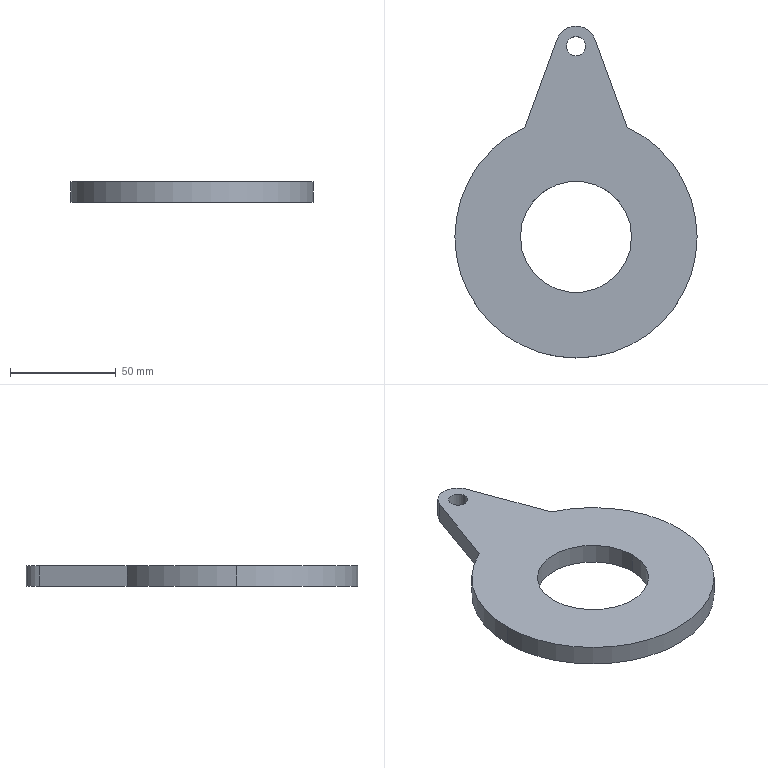Part | SolidWorks | features Extrusion 1 | 1 solid | 12 faces | box 114.3 x 156.675 x 9.525 mm | volume 88657 mm3 | cylinder 8 | plane 4 | commonest cylinder face diameters 114.3 x3 9 x2 52.502 x2 19.05 x1
STEP:
#1=CARTESIAN_POINT('',(-4.5,90.,231.775));
#2=VERTEX_POINT('',#1);
#3=CARTESIAN_POINT('',(4.5,90.,231.775));
#4=VERTEX_POINT('',#3);
#5=CARTESIAN_POINT('',(0.,90.,231.775));
#6=DIRECTION('',(0.,0.,1.));
#7=DIRECTION('',(1.,0.,0.));
#8=AXIS2_PLACEMENT_3D('',#5,#6,#7);
#9=CIRCLE('',#8,4.5);
#10=EDGE_CURVE('',#2,#4,#9,.T.);
#11=ORIENTED_EDGE('',*,*,#10,.T.);
#12=CARTESIAN_POINT('',(4.5,90.,222.25));
#13=VERTEX_POINT('',#12);
#14=CARTESIAN_POINT('',(4.5,90.,231.775));
#15=DIRECTION('',(0.,0.,-1.));
#16=VECTOR('',#15,1000.);
#17=LINE('',#14,#16);
#18=EDGE_CURVE('',#4,#13,#17,.T.);
#19=ORIENTED_EDGE('',*,*,#18,.T.);
#20=CARTESIAN_POINT('',(-4.5,90.,222.25));
#21=VERTEX_POINT('',#20);
#22=CARTESIAN_POINT('',(0.,90.,222.25));
#23=DIRECTION('',(0.,0.,1.));
#24=DIRECTION('',(1.,0.,0.));
#25=AXIS2_PLACEMENT_3D('',#22,#23,#24);
#26=CIRCLE('',#25,4.5);
#27=EDGE_CURVE('',#21,#13,#26,.T.);
#28=ORIENTED_EDGE('',*,*,#27,.F.);
#29=CARTESIAN_POINT('',(-4.5,90.,231.775));
#30=DIRECTION('',(0.,0.,-1.));
#31=VECTOR('',#30,1000.);
#32=LINE('',#29,#31);
#33=EDGE_CURVE('',#2,#21,#32,.T.);
#34=ORIENTED_EDGE('',*,*,#33,.F.);
#35=EDGE_LOOP('',(#11,#19,#28,#34));
#36=FACE_OUTER_BOUND('',#35,.T.);
#37=CARTESIAN_POINT('',(0.,90.,231.775));
#38=DIRECTION('',(0.,0.,-1.));
#39=DIRECTION('',(-1.,0.,0.));
#40=AXIS2_PLACEMENT_3D('',#37,#38,#39);
#41=CYLINDRICAL_SURFACE('',#40,4.5);
#42=ADVANCED_FACE('',(#36),#41,.F.);
#43=CARTESIAN_POINT('',(-26.251,0.,231.775));
#44=VERTEX_POINT('',#43);
#45=CARTESIAN_POINT('',(26.251,0.,231.775));
#46=VERTEX_POINT('',#45);
#47=CARTESIAN_POINT('',(0.,0.,231.775));
#48=DIRECTION('',(0.,0.,1.));
#49=DIRECTION('',(1.,0.,0.));
#50=AXIS2_PLACEMENT_3D('',#47,#48,#49);
#51=CIRCLE('',#50,26.251);
#52=EDGE_CURVE('',#44,#46,#51,.T.);
#53=ORIENTED_EDGE('',*,*,#52,.T.);
#54=CARTESIAN_POINT('',(26.251,0.,222.25));
#55=VERTEX_POINT('',#54);
#56=CARTESIAN_POINT('',(26.251,0.,231.775));
#57=DIRECTION('',(0.,0.,-1.));
#58=VECTOR('',#57,1000.);
#59=LINE('',#56,#58);
#60=EDGE_CURVE('',#46,#55,#59,.T.);
#61=ORIENTED_EDGE('',*,*,#60,.T.);
#62=CARTESIAN_POINT('',(-26.251,0.,222.25));
#63=VERTEX_POINT('',#62);
#64=CARTESIAN_POINT('',(0.,0.,222.25));
#65=DIRECTION('',(0.,0.,1.));
#66=DIRECTION('',(1.,0.,0.));
#67=AXIS2_PLACEMENT_3D('',#64,#65,#66);
#68=CIRCLE('',#67,26.251);
#69=EDGE_CURVE('',#63,#55,#68,.T.);
#70=ORIENTED_EDGE('',*,*,#69,.F.);
#71=CARTESIAN_POINT('',(-26.251,0.,231.775));
#72=DIRECTION('',(0.,0.,-1.));
#73=VECTOR('',#72,1000.);
#74=LINE('',#71,#73);
#75=EDGE_CURVE('',#44,#63,#74,.T.);
#76=ORIENTED_EDGE('',*,*,#75,.F.);
#77=EDGE_LOOP('',(#53,#61,#70,#76));
#78=FACE_OUTER_BOUND('',#77,.T.);
#79=CARTESIAN_POINT('',(0.,0.,231.775));
#80=DIRECTION('',(0.,0.,-1.));
#81=DIRECTION('',(-1.,0.,0.));
#82=AXIS2_PLACEMENT_3D('',#79,#80,#81);
#83=CYLINDRICAL_SURFACE('',#82,26.251);
#84=ADVANCED_FACE('',(#78),#83,.F.);
#85=CARTESIAN_POINT('',(57.15,0.,231.775));
#86=VERTEX_POINT('',#85);
#87=CARTESIAN_POINT('',(24.019,51.858,231.775));
#88=VERTEX_POINT('',#87);
#89=CARTESIAN_POINT('',(0.,0.,231.775));
#90=DIRECTION('',(0.,0.,1.));
#91=DIRECTION('',(1.,0.,0.));
#92=AXIS2_PLACEMENT_3D('',#89,#90,#91);
#93=CIRCLE('',#92,57.15);
#94=EDGE_CURVE('',#86,#88,#93,.T.);
#95=ORIENTED_EDGE('',*,*,#94,.F.);
#96=CARTESIAN_POINT('',(57.15,0.,222.25));
#97=VERTEX_POINT('',#96);
#98=CARTESIAN_POINT('',(57.15,0.,231.775));
#99=DIRECTION('',(0.,0.,-1.));
#100=VECTOR('',#99,1000.);
#101=LINE('',#98,#100);
#102=EDGE_CURVE('',#86,#97,#101,.T.);
#103=ORIENTED_EDGE('',*,*,#102,.T.);
#104=CARTESIAN_POINT('',(24.019,51.858,222.25));
#105=VERTEX_POINT('',#104);
#106=CARTESIAN_POINT('',(0.,0.,222.25));
#107=DIRECTION('',(0.,0.,1.));
#108=DIRECTION('',(1.,0.,0.));
#109=AXIS2_PLACEMENT_3D('',#106,#107,#108);
#110=CIRCLE('',#109,57.15);
#111=EDGE_CURVE('',#97,#105,#110,.T.);
#112=ORIENTED_EDGE('',*,*,#111,.T.);
#113=CARTESIAN_POINT('',(24.019,51.858,231.775));
#114=DIRECTION('',(0.,0.,-1.));
#115=VECTOR('',#114,1000.);
#116=LINE('',#113,#115);
#117=EDGE_CURVE('',#88,#105,#116,.T.);
#118=ORIENTED_EDGE('',*,*,#117,.F.);
#119=EDGE_LOOP('',(#95,#103,#112,#118));
#120=FACE_OUTER_BOUND('',#119,.T.);
#121=CARTESIAN_POINT('',(0.,0.,231.775));
#122=DIRECTION('',(0.,0.,-1.));
#123=DIRECTION('',(-1.,0.,0.));
#124=AXIS2_PLACEMENT_3D('',#121,#122,#123);
#125=CYLINDRICAL_SURFACE('',#124,57.15);
#126=ADVANCED_FACE('',(#120),#125,.T.);
#127=ORIENTED_EDGE('',*,*,#102,.F.);
#128=CARTESIAN_POINT('',(-57.15,0.,231.775));
#129=VERTEX_POINT('',#128);
#130=CARTESIAN_POINT('',(0.,0.,231.775));
#131=DIRECTION('',(0.,0.,1.));
#132=DIRECTION('',(1.,0.,0.));
#133=AXIS2_PLACEMENT_3D('',#130,#131,#132);
#134=CIRCLE('',#133,57.15);
#135=EDGE_CURVE('',#129,#86,#134,.T.);
#136=ORIENTED_EDGE('',*,*,#135,.F.);
#137=CARTESIAN_POINT('',(-57.15,0.,222.25));
#138=VERTEX_POINT('',#137);
#139=CARTESIAN_POINT('',(-57.15,0.,231.775));
#140=DIRECTION('',(0.,0.,-1.));
#141=VECTOR('',#140,1000.);
#142=LINE('',#139,#141);
#143=EDGE_CURVE('',#129,#138,#142,.T.);
#144=ORIENTED_EDGE('',*,*,#143,.T.);
#145=CARTESIAN_POINT('',(0.,0.,222.25));
#146=DIRECTION('',(0.,0.,1.));
#147=DIRECTION('',(1.,0.,0.));
#148=AXIS2_PLACEMENT_3D('',#145,#146,#147);
#149=CIRCLE('',#148,57.15);
#150=EDGE_CURVE('',#138,#97,#149,.T.);
#151=ORIENTED_EDGE('',*,*,#150,.T.);
#152=EDGE_LOOP('',(#127,#136,#144,#151));
#153=FACE_OUTER_BOUND('',#152,.T.);
#154=CARTESIAN_POINT('',(0.,0.,231.775));
#155=DIRECTION('',(0.,0.,-1.));
#156=DIRECTION('',(-1.,0.,0.));
#157=AXIS2_PLACEMENT_3D('',#154,#155,#156);
#158=CYLINDRICAL_SURFACE('',#157,57.15);
#159=ADVANCED_FACE('',(#153),#158,.T.);
#160=ORIENTED_EDGE('',*,*,#52,.F.);
#161=CARTESIAN_POINT('',(0.,0.,231.775));
#162=DIRECTION('',(0.,0.,1.));
#163=DIRECTION('',(1.,0.,0.));
#164=AXIS2_PLACEMENT_3D('',#161,#162,#163);
#165=CIRCLE('',#164,26.251);
#166=EDGE_CURVE('',#46,#44,#165,.T.);
#167=ORIENTED_EDGE('',*,*,#166,.F.);
#168=EDGE_LOOP('',(#160,#167));
#169=FACE_BOUND('',#168,.T.);
#170=CARTESIAN_POINT('',(8.951,93.258,231.775));
#171=VERTEX_POINT('',#170);
#172=CARTESIAN_POINT('',(-8.951,93.258,231.775));
#173=VERTEX_POINT('',#172);
#174=CARTESIAN_POINT('',(0.,90.,231.775));
#175=DIRECTION('',(0.,0.,1.));
#176=DIRECTION('',(1.,0.,0.));
#177=AXIS2_PLACEMENT_3D('',#174,#175,#176);
#178=CIRCLE('',#177,9.525);
#179=EDGE_CURVE('',#171,#173,#178,.T.);
#180=ORIENTED_EDGE('',*,*,#179,.T.);
#181=CARTESIAN_POINT('',(-24.019,51.858,231.775));
#182=VERTEX_POINT('',#181);
#183=CARTESIAN_POINT('',(-8.951,93.258,231.775));
#184=DIRECTION('',(-0.342,-0.9397,0.));
#185=VECTOR('',#184,1000.);
#186=LINE('',#183,#185);
#187=EDGE_CURVE('',#173,#182,#186,.T.);
#188=ORIENTED_EDGE('',*,*,#187,.T.);
#189=CARTESIAN_POINT('',(0.,0.,231.775));
#190=DIRECTION('',(0.,0.,1.));
#191=DIRECTION('',(1.,0.,0.));
#192=AXIS2_PLACEMENT_3D('',#189,#190,#191);
#193=CIRCLE('',#192,57.15);
#194=EDGE_CURVE('',#182,#129,#193,.T.);
#195=ORIENTED_EDGE('',*,*,#194,.T.);
#196=ORIENTED_EDGE('',*,*,#135,.T.);
#197=ORIENTED_EDGE('',*,*,#94,.T.);
#198=CARTESIAN_POINT('',(8.951,93.258,231.775));
#199=DIRECTION('',(-0.342,0.9397,0.));
#200=VECTOR('',#199,1000.);
#201=LINE('',#198,#200);
#202=EDGE_CURVE('',#88,#171,#201,.T.);
#203=ORIENTED_EDGE('',*,*,#202,.T.);
#204=EDGE_LOOP('',(#180,#188,#195,#196,#197,#203));
#205=FACE_OUTER_BOUND('',#204,.T.);
#206=ORIENTED_EDGE('',*,*,#10,.F.);
#207=CARTESIAN_POINT('',(0.,90.,231.775));
#208=DIRECTION('',(0.,0.,1.));
#209=DIRECTION('',(1.,0.,0.));
#210=AXIS2_PLACEMENT_3D('',#207,#208,#209);
#211=CIRCLE('',#210,4.5);
#212=EDGE_CURVE('',#4,#2,#211,.T.);
#213=ORIENTED_EDGE('',*,*,#212,.F.);
#214=EDGE_LOOP('',(#206,#213));
#215=FACE_BOUND('',#214,.T.);
#216=CARTESIAN_POINT('',(0.,90.,231.775));
#217=DIRECTION('',(0.,0.,1.));
#218=DIRECTION('',(1.,0.,0.));
#219=AXIS2_PLACEMENT_3D('',#216,#217,#218);
#220=PLANE('',#219);
#221=ADVANCED_FACE('',(#169,#205,#215),#220,.T.);
#222=CARTESIAN_POINT('',(8.951,93.258,222.25));
#223=VERTEX_POINT('',#222);
#224=CARTESIAN_POINT('',(-8.951,93.258,222.25));
#225=VERTEX_POINT('',#224);
#226=CARTESIAN_POINT('',(0.,90.,222.25));
#227=DIRECTION('',(0.,0.,1.));
#228=DIRECTION('',(1.,0.,0.));
#229=AXIS2_PLACEMENT_3D('',#226,#227,#228);
#230=CIRCLE('',#229,9.525);
#231=EDGE_CURVE('',#223,#225,#230,.T.);
#232=ORIENTED_EDGE('',*,*,#231,.F.);
#233=CARTESIAN_POINT('',(8.951,93.258,222.25));
#234=DIRECTION('',(-0.342,0.9397,0.));
#235=VECTOR('',#234,1000.);
#236=LINE('',#233,#235);
#237=EDGE_CURVE('',#105,#223,#236,.T.);
#238=ORIENTED_EDGE('',*,*,#237,.F.);
#239=ORIENTED_EDGE('',*,*,#111,.F.);
#240=ORIENTED_EDGE('',*,*,#150,.F.);
#241=CARTESIAN_POINT('',(-24.019,51.858,222.25));
#242=VERTEX_POINT('',#241);
#243=CARTESIAN_POINT('',(0.,0.,222.25));
#244=DIRECTION('',(0.,0.,1.));
#245=DIRECTION('',(1.,0.,0.));
#246=AXIS2_PLACEMENT_3D('',#243,#244,#245);
#247=CIRCLE('',#246,57.15);
#248=EDGE_CURVE('',#242,#138,#247,.T.);
#249=ORIENTED_EDGE('',*,*,#248,.F.);
#250=CARTESIAN_POINT('',(-8.951,93.258,222.25));
#251=DIRECTION('',(-0.342,-0.9397,0.));
#252=VECTOR('',#251,1000.);
#253=LINE('',#250,#252);
#254=EDGE_CURVE('',#225,#242,#253,.T.);
#255=ORIENTED_EDGE('',*,*,#254,.F.);
#256=EDGE_LOOP('',(#232,#238,#239,#240,#249,#255));
#257=FACE_OUTER_BOUND('',#256,.T.);
#258=ORIENTED_EDGE('',*,*,#69,.T.);
#259=CARTESIAN_POINT('',(0.,0.,222.25));
#260=DIRECTION('',(0.,0.,1.));
#261=DIRECTION('',(1.,0.,0.));
#262=AXIS2_PLACEMENT_3D('',#259,#260,#261);
#263=CIRCLE('',#262,26.251);
#264=EDGE_CURVE('',#55,#63,#263,.T.);
#265=ORIENTED_EDGE('',*,*,#264,.T.);
#266=EDGE_LOOP('',(#258,#265));
#267=FACE_BOUND('',#266,.T.);
#268=ORIENTED_EDGE('',*,*,#27,.T.);
#269=CARTESIAN_POINT('',(0.,90.,222.25));
#270=DIRECTION('',(0.,0.,1.));
#271=DIRECTION('',(1.,0.,0.));
#272=AXIS2_PLACEMENT_3D('',#269,#270,#271);
#273=CIRCLE('',#272,4.5);
#274=EDGE_CURVE('',#13,#21,#273,.T.);
#275=ORIENTED_EDGE('',*,*,#274,.T.);
#276=EDGE_LOOP('',(#268,#275));
#277=FACE_BOUND('',#276,.T.);
#278=CARTESIAN_POINT('',(0.,90.,222.25));
#279=DIRECTION('',(0.,0.,1.));
#280=DIRECTION('',(1.,0.,0.));
#281=AXIS2_PLACEMENT_3D('',#278,#279,#280);
#282=PLANE('',#281);
#283=ADVANCED_FACE('',(#257,#267,#277),#282,.F.);
#284=ORIENTED_EDGE('',*,*,#231,.T.);
#285=CARTESIAN_POINT('',(-8.951,93.258,231.775));
#286=DIRECTION('',(0.,0.,-1.));
#287=VECTOR('',#286,1000.);
#288=LINE('',#285,#287);
#289=EDGE_CURVE('',#173,#225,#288,.T.);
#290=ORIENTED_EDGE('',*,*,#289,.F.);
#291=ORIENTED_EDGE('',*,*,#179,.F.);
#292=CARTESIAN_POINT('',(8.951,93.258,231.775));
#293=DIRECTION('',(0.,0.,-1.));
#294=VECTOR('',#293,1000.);
#295=LINE('',#292,#294);
#296=EDGE_CURVE('',#171,#223,#295,.T.);
#297=ORIENTED_EDGE('',*,*,#296,.T.);
#298=EDGE_LOOP('',(#284,#290,#291,#297));
#299=FACE_OUTER_BOUND('',#298,.T.);
#300=CARTESIAN_POINT('',(0.,90.,231.775));
#301=DIRECTION('',(0.,0.,-1.));
#302=DIRECTION('',(-1.,0.,0.));
#303=AXIS2_PLACEMENT_3D('',#300,#301,#302);
#304=CYLINDRICAL_SURFACE('',#303,9.525);
#305=ADVANCED_FACE('',(#299),#304,.T.);
#306=ORIENTED_EDGE('',*,*,#254,.T.);
#307=CARTESIAN_POINT('',(-24.019,51.858,231.775));
#308=DIRECTION('',(0.,0.,-1.));
#309=VECTOR('',#308,1000.);
#310=LINE('',#307,#309);
#311=EDGE_CURVE('',#182,#242,#310,.T.);
#312=ORIENTED_EDGE('',*,*,#311,.F.);
#313=ORIENTED_EDGE('',*,*,#187,.F.);
#314=ORIENTED_EDGE('',*,*,#289,.T.);
#315=EDGE_LOOP('',(#306,#312,#313,#314));
#316=FACE_OUTER_BOUND('',#315,.T.);
#317=CARTESIAN_POINT('',(-8.951,93.258,231.775));
#318=DIRECTION('',(0.9397,-0.342,0.));
#319=DIRECTION('',(0.342,0.9397,0.));
#320=AXIS2_PLACEMENT_3D('',#317,#318,#319);
#321=PLANE('',#320);
#322=ADVANCED_FACE('',(#316),#321,.F.);
#323=ORIENTED_EDGE('',*,*,#143,.F.);
#324=ORIENTED_EDGE('',*,*,#194,.F.);
#325=ORIENTED_EDGE('',*,*,#311,.T.);
#326=ORIENTED_EDGE('',*,*,#248,.T.);
#327=EDGE_LOOP('',(#323,#324,#325,#326));
#328=FACE_OUTER_BOUND('',#327,.T.);
#329=CARTESIAN_POINT('',(0.,0.,231.775));
#330=DIRECTION('',(0.,0.,-1.));
#331=DIRECTION('',(-1.,0.,0.));
#332=AXIS2_PLACEMENT_3D('',#329,#330,#331);
#333=CYLINDRICAL_SURFACE('',#332,57.15);
#334=ADVANCED_FACE('',(#328),#333,.T.);
#335=ORIENTED_EDGE('',*,*,#237,.T.);
#336=ORIENTED_EDGE('',*,*,#296,.F.);
#337=ORIENTED_EDGE('',*,*,#202,.F.);
#338=ORIENTED_EDGE('',*,*,#117,.T.);
#339=EDGE_LOOP('',(#335,#336,#337,#338));
#340=FACE_OUTER_BOUND('',#339,.T.);
#341=CARTESIAN_POINT('',(8.951,93.258,231.775));
#342=DIRECTION('',(-0.9397,-0.342,0.));
#343=DIRECTION('',(0.342,-0.9397,0.));
#344=AXIS2_PLACEMENT_3D('',#341,#342,#343);
#345=PLANE('',#344);
#346=ADVANCED_FACE('',(#340),#345,.F.);
#347=ORIENTED_EDGE('',*,*,#60,.F.);
#348=ORIENTED_EDGE('',*,*,#166,.T.);
#349=ORIENTED_EDGE('',*,*,#75,.T.);
#350=ORIENTED_EDGE('',*,*,#264,.F.);
#351=EDGE_LOOP('',(#347,#348,#349,#350));
#352=FACE_OUTER_BOUND('',#351,.T.);
#353=CARTESIAN_POINT('',(0.,0.,231.775));
#354=DIRECTION('',(0.,0.,-1.));
#355=DIRECTION('',(-1.,0.,0.));
#356=AXIS2_PLACEMENT_3D('',#353,#354,#355);
#357=CYLINDRICAL_SURFACE('',#356,26.251);
#358=ADVANCED_FACE('',(#352),#357,.F.);
#359=ORIENTED_EDGE('',*,*,#18,.F.);
#360=ORIENTED_EDGE('',*,*,#212,.T.);
#361=ORIENTED_EDGE('',*,*,#33,.T.);
#362=ORIENTED_EDGE('',*,*,#274,.F.);
#363=EDGE_LOOP('',(#359,#360,#361,#362));
#364=FACE_OUTER_BOUND('',#363,.T.);
#365=CARTESIAN_POINT('',(0.,90.,231.775));
#366=DIRECTION('',(0.,0.,-1.));
#367=DIRECTION('',(-1.,0.,0.));
#368=AXIS2_PLACEMENT_3D('',#365,#366,#367);
#369=CYLINDRICAL_SURFACE('',#368,4.5);
#370=ADVANCED_FACE('',(#364),#369,.F.);
#371=CLOSED_SHELL('',(#42,#84,#126,#159,#221,#283,#305,#322,#334,#346,#358,#370));
#372=MANIFOLD_SOLID_BREP('',#371);
#373=CARTESIAN_POINT('',(0.,0.,0.));
#374=DIRECTION('',(0.,0.,1.));
#375=DIRECTION('',(1.,0.,0.));
#376=AXIS2_PLACEMENT_3D('',#373,#374,#375);
#377=(LENGTH_UNIT()NAMED_UNIT(*)SI_UNIT(.MILLI.,.METRE.));
#378=UNCERTAINTY_MEASURE_WITH_UNIT(LENGTH_MEASURE(0.00001),#377,'','');
#379=(NAMED_UNIT(*)PLANE_ANGLE_UNIT()SI_UNIT($,.RADIAN.));
#380=(NAMED_UNIT(*)SI_UNIT($,.STERADIAN.)SOLID_ANGLE_UNIT());
#381=(GEOMETRIC_REPRESENTATION_CONTEXT(3)GLOBAL_UNCERTAINTY_ASSIGNED_CONTEXT((#378))GLOBAL_UNIT_ASSIGNED_CONTEXT((#377,#379,#380))REPRESENTATION_CONTEXT('',''));
#382=ADVANCED_BREP_SHAPE_REPRESENTATION('',(#372,#376),#381);